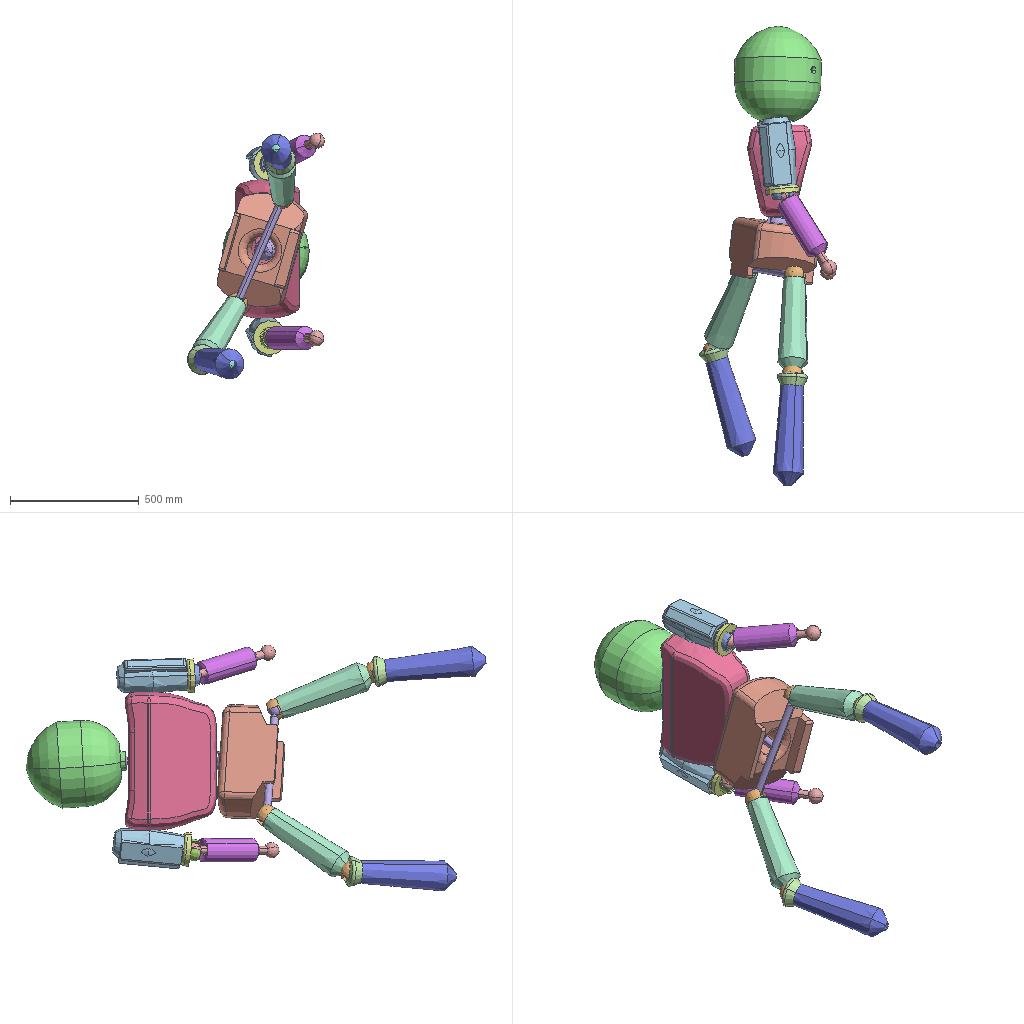Assembly | SolidWorks | 8 different items | 12 placed | box 531 x 1784 x 953 mm
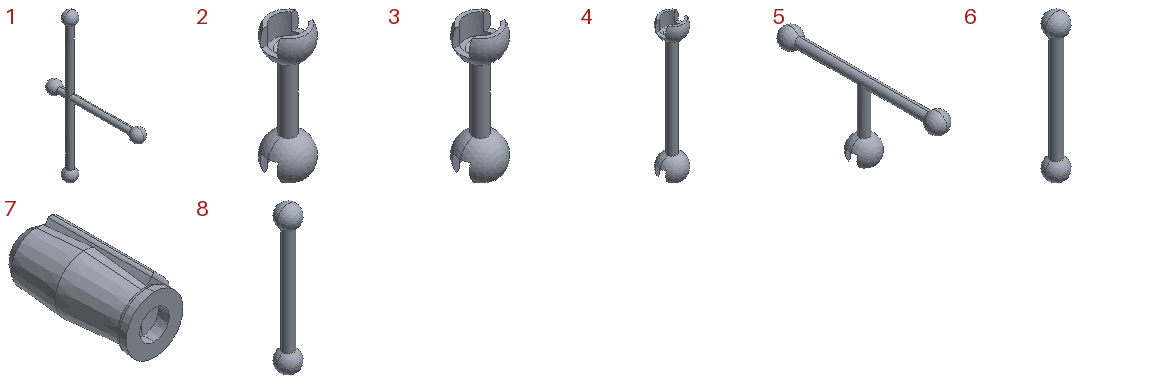Parts list (item | quantity | size | volume | features):
1 | x1 | 60 x 460 x 710 mm | 1097313 mm3 | features Revolution 3, ICE 2, Extrusion 1, MirrorPattern 1
2 | x1 | 80.921 x 85 x 255.451 mm | 326390 mm3 | features Chamfer 2, ICE 2, Extrusion 1, MirrorPattern 1, RevCut 1, Revolution 1
3 | x1 | 80.921 x 85 x 255.451 mm | 326390 mm3 | features Chamfer 2, ICE 2, Extrusion 1, MirrorPattern 1, RevCut 1, Revolution 1
4 | x2 | 80.921 x 85 x 459.451 mm | 470589 mm3 | features ICE 3, Chamfer 2, Extrusion 1, MirrorPattern 1, RevCut 1, Revolution 1
5 | x1 | 80.921 x 510 x 239.694 mm | 716291 mm3 | features ICE 3, Chamfer 2, Revolution 2, Extrusion 1, MirrorPattern 1, RevCut 1
6 | x2 | 60 x 60 x 410 mm | 433957 mm3 | features Extrusion 1, MirrorPattern 1, Revolution 1
7 | x2 | 133.247 x 297.006 x 136.186 mm | 3477471 mm3 | features Revolution 2, Fillet 1, ICE 1
8 | x2 | 60 x 60 x 410 mm | 433957 mm3 | features Extrusion 1, MirrorPattern 1, Revolution 1
Mates (type | each side: item.copy, entity, surface, feature):
Concentric | 2.1 face sphere Revolve1 | 1.1 face sphere Mirror1
Concentric | 3.1 face sphere Mirror1 | 1.1 face sphere Revolve1
Concentric | 8.1 face sphere Revolve1 | 2.1 face sphere Mirror1
Concentric | 3.1 face sphere Revolve1 | 8.2 face sphere Mirror1
Concentric | 1.1 face sphere Revolve3 | 5.1 face sphere Revolve1
Concentric | 4.1 face sphere Revolve1 | 5.1 face sphere Revolve2
Concentric | 6.1 face sphere Mirror1 | 4.1 face sphere Mirror5
Concentric | 4.2 face sphere Mirror5 | 6.2 face sphere Mirror1
Concentric | 5.1 face sphere Mirror1 | 4.2 face sphere Revolve1
Coincident | 1.1 plane | assembly plane | 3 times
Concentric | 2.1 face cylinder Boss-Extrude1 | 7.1 face cone Revolve2
Concentric | 3.1 face cylinder Boss-Extrude1 | 7.2 face cone Revolve1
Lock | 3.1 select_type:0 | 7.2 select_type:0
Lock | 2.1 select_type:0 | 7.1 select_type:0
Concentric | 6.1 face sphere Revolve1 | assembly face
Concentric | 6.2 face sphere Revolve1 | assembly face